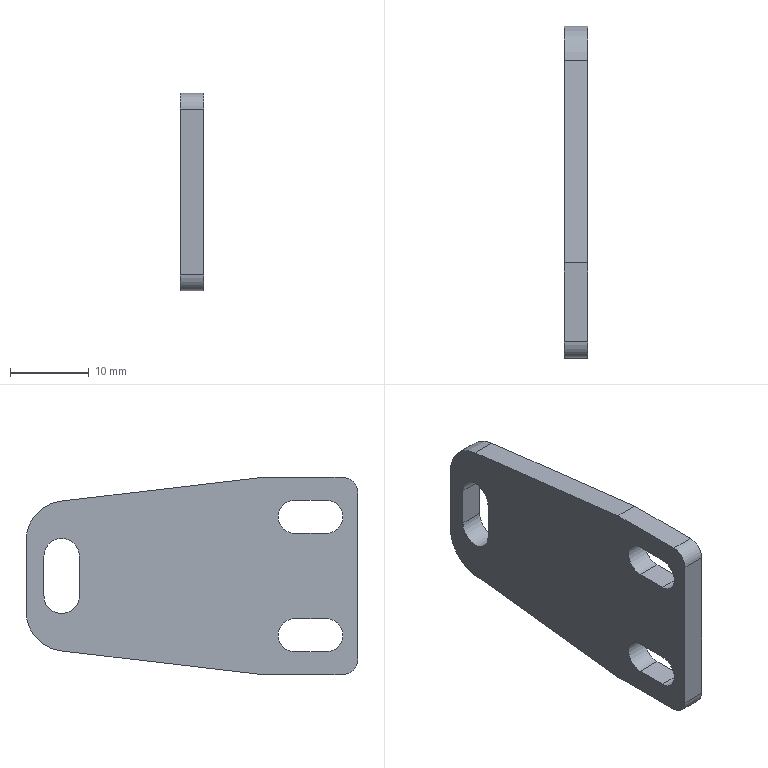Part | SolidWorks | features Fillet 3, ICE 3, Cut 1, Extrusion 1, HoleWzd 1 | 1 solid | 25 faces | box 3 x 42 x 25 mm | volume 2502 mm3 | plane 14 | cylinder 11 | commonest cylinder face diameters 4.2 x4 4.5 x3 4 x2 10 x2
STEP:
#1=CARTESIAN_POINT('',(3.,33.75,2.5));
#2=VERTEX_POINT('',#1);
#3=CARTESIAN_POINT('',(3.,31.5,4.75));
#4=VERTEX_POINT('',#3);
#5=CARTESIAN_POINT('',(3.,31.5,2.5));
#6=DIRECTION('',(1.,0.,0.));
#7=DIRECTION('',(0.,0.,-1.));
#8=AXIS2_PLACEMENT_3D('',#5,#6,#7);
#9=CIRCLE('',#8,2.25);
#10=EDGE_CURVE('',#2,#4,#9,.T.);
#11=ORIENTED_EDGE('',*,*,#10,.T.);
#12=CARTESIAN_POINT('',(0.,31.5,4.75));
#13=VERTEX_POINT('',#12);
#14=CARTESIAN_POINT('',(10.,31.5,4.75));
#15=DIRECTION('',(-1.,0.,0.));
#16=VECTOR('',#15,1000.);
#17=LINE('',#14,#16);
#18=EDGE_CURVE('',#4,#13,#17,.T.);
#19=ORIENTED_EDGE('',*,*,#18,.T.);
#20=CARTESIAN_POINT('',(0.,33.75,2.5));
#21=VERTEX_POINT('',#20);
#22=CARTESIAN_POINT('',(0.,31.5,2.5));
#23=DIRECTION('',(-1.,0.,0.));
#24=DIRECTION('',(0.,0.,1.));
#25=AXIS2_PLACEMENT_3D('',#22,#23,#24);
#26=CIRCLE('',#25,2.25);
#27=EDGE_CURVE('',#13,#21,#26,.T.);
#28=ORIENTED_EDGE('',*,*,#27,.T.);
#29=CARTESIAN_POINT('',(10.,33.75,2.5));
#30=DIRECTION('',(-1.,0.,0.));
#31=VECTOR('',#30,1000.);
#32=LINE('',#29,#31);
#33=EDGE_CURVE('',#2,#21,#32,.T.);
#34=ORIENTED_EDGE('',*,*,#33,.F.);
#35=EDGE_LOOP('',(#11,#19,#28,#34));
#36=FACE_OUTER_BOUND('',#35,.T.);
#37=CARTESIAN_POINT('',(10.,31.5,2.5));
#38=DIRECTION('',(-1.,0.,0.));
#39=DIRECTION('',(0.,0.,1.));
#40=AXIS2_PLACEMENT_3D('',#37,#38,#39);
#41=CYLINDRICAL_SURFACE('',#40,2.25);
#42=ADVANCED_FACE('',(#36),#41,.F.);
#43=CARTESIAN_POINT('',(0.,29.25,-2.5));
#44=VERTEX_POINT('',#43);
#45=CARTESIAN_POINT('',(0.,29.25,2.5));
#46=VERTEX_POINT('',#45);
#47=CARTESIAN_POINT('',(0.,29.25,-2.5));
#48=DIRECTION('',(0.,0.,1.));
#49=VECTOR('',#48,1000.);
#50=LINE('',#47,#49);
#51=EDGE_CURVE('',#44,#46,#50,.T.);
#52=ORIENTED_EDGE('',*,*,#51,.F.);
#53=CARTESIAN_POINT('',(0.,33.75,-2.5));
#54=VERTEX_POINT('',#53);
#55=CARTESIAN_POINT('',(0.,31.5,-2.5));
#56=DIRECTION('',(-1.,0.,0.));
#57=DIRECTION('',(0.,0.,1.));
#58=AXIS2_PLACEMENT_3D('',#55,#56,#57);
#59=CIRCLE('',#58,2.25);
#60=EDGE_CURVE('',#54,#44,#59,.T.);
#61=ORIENTED_EDGE('',*,*,#60,.F.);
#62=CARTESIAN_POINT('',(0.,33.75,-2.5));
#63=DIRECTION('',(0.,0.,-1.));
#64=VECTOR('',#63,1000.);
#65=LINE('',#62,#64);
#66=EDGE_CURVE('',#21,#54,#65,.T.);
#67=ORIENTED_EDGE('',*,*,#66,.F.);
#68=ORIENTED_EDGE('',*,*,#27,.F.);
#69=CARTESIAN_POINT('',(0.,31.5,2.5));
#70=DIRECTION('',(-1.,0.,0.));
#71=DIRECTION('',(0.,0.,1.));
#72=AXIS2_PLACEMENT_3D('',#69,#70,#71);
#73=CIRCLE('',#72,2.25);
#74=EDGE_CURVE('',#46,#13,#73,.T.);
#75=ORIENTED_EDGE('',*,*,#74,.F.);
#76=EDGE_LOOP('',(#52,#61,#67,#68,#75));
#77=FACE_BOUND('',#76,.T.);
#78=CARTESIAN_POINT('',(0.,2.,5.4));
#79=VERTEX_POINT('',#78);
#80=CARTESIAN_POINT('',(0.,-2.,5.4));
#81=VERTEX_POINT('',#80);
#82=CARTESIAN_POINT('',(0.,2.,5.4));
#83=DIRECTION('',(0.,-1.,0.));
#84=VECTOR('',#83,1000.);
#85=LINE('',#82,#84);
#86=EDGE_CURVE('',#79,#81,#85,.T.);
#87=ORIENTED_EDGE('',*,*,#86,.F.);
#88=CARTESIAN_POINT('',(0.,2.,9.6));
#89=VERTEX_POINT('',#88);
#90=CARTESIAN_POINT('',(0.,2.,7.5));
#91=DIRECTION('',(-1.,0.,0.));
#92=DIRECTION('',(0.,0.,-1.));
#93=AXIS2_PLACEMENT_3D('',#90,#91,#92);
#94=CIRCLE('',#93,2.1);
#95=EDGE_CURVE('',#89,#79,#94,.T.);
#96=ORIENTED_EDGE('',*,*,#95,.F.);
#97=CARTESIAN_POINT('',(0.,-2.,9.6));
#98=VERTEX_POINT('',#97);
#99=CARTESIAN_POINT('',(0.,2.,9.6));
#100=DIRECTION('',(0.,1.,0.));
#101=VECTOR('',#100,1000.);
#102=LINE('',#99,#101);
#103=EDGE_CURVE('',#98,#89,#102,.T.);
#104=ORIENTED_EDGE('',*,*,#103,.F.);
#105=CARTESIAN_POINT('',(0.,-2.,7.5));
#106=DIRECTION('',(-1.,0.,0.));
#107=DIRECTION('',(0.,0.,-1.));
#108=AXIS2_PLACEMENT_3D('',#105,#106,#107);
#109=CIRCLE('',#108,2.1);
#110=EDGE_CURVE('',#81,#98,#109,.T.);
#111=ORIENTED_EDGE('',*,*,#110,.F.);
#112=EDGE_LOOP('',(#87,#96,#104,#111));
#113=FACE_BOUND('',#112,.T.);
#114=CARTESIAN_POINT('',(0.,2.,-9.6));
#115=VERTEX_POINT('',#114);
#116=CARTESIAN_POINT('',(0.,-2.,-9.6));
#117=VERTEX_POINT('',#116);
#118=CARTESIAN_POINT('',(0.,2.,-9.6));
#119=DIRECTION('',(0.,-1.,0.));
#120=VECTOR('',#119,1000.);
#121=LINE('',#118,#120);
#122=EDGE_CURVE('',#115,#117,#121,.T.);
#123=ORIENTED_EDGE('',*,*,#122,.F.);
#124=CARTESIAN_POINT('',(0.,2.,-5.4));
#125=VERTEX_POINT('',#124);
#126=CARTESIAN_POINT('',(0.,2.,-7.5));
#127=DIRECTION('',(-1.,0.,0.));
#128=DIRECTION('',(0.,0.,1.));
#129=AXIS2_PLACEMENT_3D('',#126,#127,#128);
#130=CIRCLE('',#129,2.1);
#131=EDGE_CURVE('',#125,#115,#130,.T.);
#132=ORIENTED_EDGE('',*,*,#131,.F.);
#133=CARTESIAN_POINT('',(0.,-2.,-5.4));
#134=VERTEX_POINT('',#133);
#135=CARTESIAN_POINT('',(0.,2.,-5.4));
#136=DIRECTION('',(0.,1.,0.));
#137=VECTOR('',#136,1000.);
#138=LINE('',#135,#137);
#139=EDGE_CURVE('',#134,#125,#138,.T.);
#140=ORIENTED_EDGE('',*,*,#139,.F.);
#141=CARTESIAN_POINT('',(0.,-2.,-7.5));
#142=DIRECTION('',(-1.,0.,0.));
#143=DIRECTION('',(0.,0.,1.));
#144=AXIS2_PLACEMENT_3D('',#141,#142,#143);
#145=CIRCLE('',#144,2.1);
#146=EDGE_CURVE('',#117,#134,#145,.T.);
#147=ORIENTED_EDGE('',*,*,#146,.F.);
#148=EDGE_LOOP('',(#123,#132,#140,#147));
#149=FACE_BOUND('',#148,.T.);
#150=CARTESIAN_POINT('',(0.,36.,4.511));
#151=VERTEX_POINT('',#150);
#152=CARTESIAN_POINT('',(0.,36.,-4.511));
#153=VERTEX_POINT('',#152);
#154=CARTESIAN_POINT('',(0.,36.,0.));
#155=DIRECTION('',(0.,0.,-1.));
#156=VECTOR('',#155,1000.);
#157=LINE('',#154,#156);
#158=EDGE_CURVE('',#151,#153,#157,.T.);
#159=ORIENTED_EDGE('',*,*,#158,.T.);
#160=CARTESIAN_POINT('',(0.,31.587,-9.476));
#161=VERTEX_POINT('',#160);
#162=CARTESIAN_POINT('',(0.,31.,-4.511));
#163=DIRECTION('',(-1.,0.,0.));
#164=DIRECTION('',(0.,0.,-1.));
#165=AXIS2_PLACEMENT_3D('',#162,#163,#164);
#166=CIRCLE('',#165,5.);
#167=EDGE_CURVE('',#153,#161,#166,.T.);
#168=ORIENTED_EDGE('',*,*,#167,.T.);
#169=CARTESIAN_POINT('',(0.,6.,-12.5));
#170=VERTEX_POINT('',#169);
#171=CARTESIAN_POINT('',(0.,61.,-6.));
#172=DIRECTION('',(0.,-0.9931,-0.1174));
#173=VECTOR('',#172,1000.);
#174=LINE('',#171,#173);
#175=EDGE_CURVE('',#161,#170,#174,.T.);
#176=ORIENTED_EDGE('',*,*,#175,.T.);
#177=CARTESIAN_POINT('',(0.,-4.,-12.5));
#178=VERTEX_POINT('',#177);
#179=CARTESIAN_POINT('',(0.,6.,-12.5));
#180=DIRECTION('',(0.,1.,0.));
#181=VECTOR('',#180,1000.);
#182=LINE('',#179,#181);
#183=EDGE_CURVE('',#178,#170,#182,.T.);
#184=ORIENTED_EDGE('',*,*,#183,.F.);
#185=CARTESIAN_POINT('',(0.,-6.,-10.5));
#186=VERTEX_POINT('',#185);
#187=CARTESIAN_POINT('',(0.,-4.,-10.5));
#188=DIRECTION('',(-1.,0.,0.));
#189=DIRECTION('',(0.,0.,-1.));
#190=AXIS2_PLACEMENT_3D('',#187,#188,#189);
#191=CIRCLE('',#190,2.);
#192=EDGE_CURVE('',#178,#186,#191,.T.);
#193=ORIENTED_EDGE('',*,*,#192,.T.);
#194=CARTESIAN_POINT('',(0.,-6.,10.5));
#195=VERTEX_POINT('',#194);
#196=CARTESIAN_POINT('',(0.,-6.,12.5));
#197=DIRECTION('',(0.,0.,-1.));
#198=VECTOR('',#197,1000.);
#199=LINE('',#196,#198);
#200=EDGE_CURVE('',#195,#186,#199,.T.);
#201=ORIENTED_EDGE('',*,*,#200,.F.);
#202=CARTESIAN_POINT('',(0.,-4.,12.5));
#203=VERTEX_POINT('',#202);
#204=CARTESIAN_POINT('',(0.,-4.,10.5));
#205=DIRECTION('',(-1.,0.,0.));
#206=DIRECTION('',(0.,0.,-1.));
#207=AXIS2_PLACEMENT_3D('',#204,#205,#206);
#208=CIRCLE('',#207,2.);
#209=EDGE_CURVE('',#195,#203,#208,.T.);
#210=ORIENTED_EDGE('',*,*,#209,.T.);
#211=CARTESIAN_POINT('',(0.,6.,12.5));
#212=VERTEX_POINT('',#211);
#213=CARTESIAN_POINT('',(0.,6.,12.5));
#214=DIRECTION('',(0.,-1.,0.));
#215=VECTOR('',#214,1000.);
#216=LINE('',#213,#215);
#217=EDGE_CURVE('',#212,#203,#216,.T.);
#218=ORIENTED_EDGE('',*,*,#217,.F.);
#219=CARTESIAN_POINT('',(0.,31.587,9.476));
#220=VERTEX_POINT('',#219);
#221=CARTESIAN_POINT('',(0.,61.,6.));
#222=DIRECTION('',(0.,0.9931,-0.1174));
#223=VECTOR('',#222,1000.);
#224=LINE('',#221,#223);
#225=EDGE_CURVE('',#212,#220,#224,.T.);
#226=ORIENTED_EDGE('',*,*,#225,.T.);
#227=CARTESIAN_POINT('',(0.,31.,4.511));
#228=DIRECTION('',(-1.,0.,0.));
#229=DIRECTION('',(0.,0.,-1.));
#230=AXIS2_PLACEMENT_3D('',#227,#228,#229);
#231=CIRCLE('',#230,5.);
#232=EDGE_CURVE('',#220,#151,#231,.T.);
#233=ORIENTED_EDGE('',*,*,#232,.T.);
#234=EDGE_LOOP('',(#159,#168,#176,#184,#193,#201,#210,#218,#226,#233));
#235=FACE_OUTER_BOUND('',#234,.T.);
#236=CARTESIAN_POINT('',(0.,0.,0.));
#237=DIRECTION('',(1.,0.,0.));
#238=DIRECTION('',(0.,0.,-1.));
#239=AXIS2_PLACEMENT_3D('',#236,#237,#238);
#240=PLANE('',#239);
#241=ADVANCED_FACE('',(#77,#113,#149,#235),#240,.F.);
#242=CARTESIAN_POINT('',(3.,-4.,-12.5));
#243=VERTEX_POINT('',#242);
#244=CARTESIAN_POINT('',(3.,6.,-12.5));
#245=VERTEX_POINT('',#244);
#246=CARTESIAN_POINT('',(3.,6.,-12.5));
#247=DIRECTION('',(0.,1.,0.));
#248=VECTOR('',#247,1000.);
#249=LINE('',#246,#248);
#250=EDGE_CURVE('',#243,#245,#249,.T.);
#251=ORIENTED_EDGE('',*,*,#250,.F.);
#252=CARTESIAN_POINT('',(3.,-4.,-12.5));
#253=DIRECTION('',(-1.,0.,0.));
#254=VECTOR('',#253,1000.);
#255=LINE('',#252,#254);
#256=EDGE_CURVE('',#243,#178,#255,.T.);
#257=ORIENTED_EDGE('',*,*,#256,.T.);
#258=ORIENTED_EDGE('',*,*,#183,.T.);
#259=CARTESIAN_POINT('',(3.,6.,-12.5));
#260=DIRECTION('',(-1.,0.,0.));
#261=VECTOR('',#260,1000.);
#262=LINE('',#259,#261);
#263=EDGE_CURVE('',#245,#170,#262,.T.);
#264=ORIENTED_EDGE('',*,*,#263,.F.);
#265=EDGE_LOOP('',(#251,#257,#258,#264));
#266=FACE_OUTER_BOUND('',#265,.T.);
#267=CARTESIAN_POINT('',(3.,6.,-12.5));
#268=DIRECTION('',(0.,0.,1.));
#269=DIRECTION('',(0.,-1.,0.));
#270=AXIS2_PLACEMENT_3D('',#267,#268,#269);
#271=PLANE('',#270);
#272=ADVANCED_FACE('',(#266),#271,.F.);
#273=ORIENTED_EDGE('',*,*,#217,.T.);
#274=CARTESIAN_POINT('',(3.,-4.,12.5));
#275=VERTEX_POINT('',#274);
#276=CARTESIAN_POINT('',(3.,-4.,12.5));
#277=DIRECTION('',(1.,0.,0.));
#278=VECTOR('',#277,1000.);
#279=LINE('',#276,#278);
#280=EDGE_CURVE('',#203,#275,#279,.T.);
#281=ORIENTED_EDGE('',*,*,#280,.T.);
#282=CARTESIAN_POINT('',(3.,6.,12.5));
#283=VERTEX_POINT('',#282);
#284=CARTESIAN_POINT('',(3.,6.,12.5));
#285=DIRECTION('',(0.,-1.,0.));
#286=VECTOR('',#285,1000.);
#287=LINE('',#284,#286);
#288=EDGE_CURVE('',#283,#275,#287,.T.);
#289=ORIENTED_EDGE('',*,*,#288,.F.);
#290=CARTESIAN_POINT('',(3.,6.,12.5));
#291=DIRECTION('',(-1.,0.,0.));
#292=VECTOR('',#291,1000.);
#293=LINE('',#290,#292);
#294=EDGE_CURVE('',#283,#212,#293,.T.);
#295=ORIENTED_EDGE('',*,*,#294,.T.);
#296=EDGE_LOOP('',(#273,#281,#289,#295));
#297=FACE_OUTER_BOUND('',#296,.T.);
#298=CARTESIAN_POINT('',(3.,6.,12.5));
#299=DIRECTION('',(0.,0.,-1.));
#300=DIRECTION('',(-1.,0.,0.));
#301=AXIS2_PLACEMENT_3D('',#298,#299,#300);
#302=PLANE('',#301);
#303=ADVANCED_FACE('',(#297),#302,.F.);
#304=ORIENTED_EDGE('',*,*,#200,.T.);
#305=CARTESIAN_POINT('',(3.,-6.,-10.5));
#306=VERTEX_POINT('',#305);
#307=CARTESIAN_POINT('',(3.,-6.,-10.5));
#308=DIRECTION('',(1.,0.,0.));
#309=VECTOR('',#308,1000.);
#310=LINE('',#307,#309);
#311=EDGE_CURVE('',#186,#306,#310,.T.);
#312=ORIENTED_EDGE('',*,*,#311,.T.);
#313=CARTESIAN_POINT('',(3.,-6.,10.5));
#314=VERTEX_POINT('',#313);
#315=CARTESIAN_POINT('',(3.,-6.,12.5));
#316=DIRECTION('',(0.,0.,-1.));
#317=VECTOR('',#316,1000.);
#318=LINE('',#315,#317);
#319=EDGE_CURVE('',#314,#306,#318,.T.);
#320=ORIENTED_EDGE('',*,*,#319,.F.);
#321=CARTESIAN_POINT('',(3.,-6.,10.5));
#322=DIRECTION('',(-1.,0.,0.));
#323=VECTOR('',#322,1000.);
#324=LINE('',#321,#323);
#325=EDGE_CURVE('',#314,#195,#324,.T.);
#326=ORIENTED_EDGE('',*,*,#325,.T.);
#327=EDGE_LOOP('',(#304,#312,#320,#326));
#328=FACE_OUTER_BOUND('',#327,.T.);
#329=CARTESIAN_POINT('',(3.,-6.,12.5));
#330=DIRECTION('',(0.,1.,0.));
#331=DIRECTION('',(0.,0.,1.));
#332=AXIS2_PLACEMENT_3D('',#329,#330,#331);
#333=PLANE('',#332);
#334=ADVANCED_FACE('',(#328),#333,.F.);
#335=CARTESIAN_POINT('',(3.,29.25,-2.5));
#336=VERTEX_POINT('',#335);
#337=CARTESIAN_POINT('',(3.,33.75,-2.5));
#338=VERTEX_POINT('',#337);
#339=CARTESIAN_POINT('',(3.,31.5,-2.5));
#340=DIRECTION('',(1.,0.,0.));
#341=DIRECTION('',(0.,0.,-1.));
#342=AXIS2_PLACEMENT_3D('',#339,#340,#341);
#343=CIRCLE('',#342,2.25);
#344=EDGE_CURVE('',#336,#338,#343,.T.);
#345=ORIENTED_EDGE('',*,*,#344,.F.);
#346=CARTESIAN_POINT('',(3.,29.25,2.5));
#347=VERTEX_POINT('',#346);
#348=CARTESIAN_POINT('',(3.,29.25,0.));
#349=DIRECTION('',(0.,0.,-1.));
#350=VECTOR('',#349,1000.);
#351=LINE('',#348,#350);
#352=EDGE_CURVE('',#347,#336,#351,.T.);
#353=ORIENTED_EDGE('',*,*,#352,.F.);
#354=CARTESIAN_POINT('',(3.,31.5,2.5));
#355=DIRECTION('',(1.,0.,0.));
#356=DIRECTION('',(0.,0.,-1.));
#357=AXIS2_PLACEMENT_3D('',#354,#355,#356);
#358=CIRCLE('',#357,2.25);
#359=EDGE_CURVE('',#4,#347,#358,.T.);
#360=ORIENTED_EDGE('',*,*,#359,.F.);
#361=ORIENTED_EDGE('',*,*,#10,.F.);
#362=CARTESIAN_POINT('',(3.,33.75,0.));
#363=DIRECTION('',(0.,0.,1.));
#364=VECTOR('',#363,1000.);
#365=LINE('',#362,#364);
#366=EDGE_CURVE('',#338,#2,#365,.T.);
#367=ORIENTED_EDGE('',*,*,#366,.F.);
#368=EDGE_LOOP('',(#345,#353,#360,#361,#367));
#369=FACE_BOUND('',#368,.T.);
#370=CARTESIAN_POINT('',(3.,31.587,-9.476));
#371=VERTEX_POINT('',#370);
#372=CARTESIAN_POINT('',(3.,61.,-6.));
#373=DIRECTION('',(0.,-0.9931,-0.1174));
#374=VECTOR('',#373,1000.);
#375=LINE('',#372,#374);
#376=EDGE_CURVE('',#371,#245,#375,.T.);
#377=ORIENTED_EDGE('',*,*,#376,.F.);
#378=CARTESIAN_POINT('',(3.,36.,-4.511));
#379=VERTEX_POINT('',#378);
#380=CARTESIAN_POINT('',(3.,31.,-4.511));
#381=DIRECTION('',(1.,0.,0.));
#382=DIRECTION('',(0.,0.,-1.));
#383=AXIS2_PLACEMENT_3D('',#380,#381,#382);
#384=CIRCLE('',#383,5.);
#385=EDGE_CURVE('',#371,#379,#384,.T.);
#386=ORIENTED_EDGE('',*,*,#385,.T.);
#387=CARTESIAN_POINT('',(3.,36.,4.511));
#388=VERTEX_POINT('',#387);
#389=CARTESIAN_POINT('',(3.,36.,13.476));
#390=DIRECTION('',(0.,0.,-1.));
#391=VECTOR('',#390,1000.);
#392=LINE('',#389,#391);
#393=EDGE_CURVE('',#388,#379,#392,.T.);
#394=ORIENTED_EDGE('',*,*,#393,.F.);
#395=CARTESIAN_POINT('',(3.,31.587,9.476));
#396=VERTEX_POINT('',#395);
#397=CARTESIAN_POINT('',(3.,31.,4.511));
#398=DIRECTION('',(1.,0.,0.));
#399=DIRECTION('',(0.,0.,-1.));
#400=AXIS2_PLACEMENT_3D('',#397,#398,#399);
#401=CIRCLE('',#400,5.);
#402=EDGE_CURVE('',#388,#396,#401,.T.);
#403=ORIENTED_EDGE('',*,*,#402,.T.);
#404=CARTESIAN_POINT('',(3.,61.,6.));
#405=DIRECTION('',(0.,0.9931,-0.1174));
#406=VECTOR('',#405,1000.);
#407=LINE('',#404,#406);
#408=EDGE_CURVE('',#283,#396,#407,.T.);
#409=ORIENTED_EDGE('',*,*,#408,.F.);
#410=ORIENTED_EDGE('',*,*,#288,.T.);
#411=CARTESIAN_POINT('',(3.,-4.,10.5));
#412=DIRECTION('',(1.,0.,0.));
#413=DIRECTION('',(0.,0.,-1.));
#414=AXIS2_PLACEMENT_3D('',#411,#412,#413);
#415=CIRCLE('',#414,2.);
#416=EDGE_CURVE('',#275,#314,#415,.T.);
#417=ORIENTED_EDGE('',*,*,#416,.T.);
#418=ORIENTED_EDGE('',*,*,#319,.T.);
#419=CARTESIAN_POINT('',(3.,-4.,-10.5));
#420=DIRECTION('',(1.,0.,0.));
#421=DIRECTION('',(0.,0.,-1.));
#422=AXIS2_PLACEMENT_3D('',#419,#420,#421);
#423=CIRCLE('',#422,2.);
#424=EDGE_CURVE('',#306,#243,#423,.T.);
#425=ORIENTED_EDGE('',*,*,#424,.T.);
#426=ORIENTED_EDGE('',*,*,#250,.T.);
#427=EDGE_LOOP('',(#377,#386,#394,#403,#409,#410,#417,#418,#425,#426));
#428=FACE_OUTER_BOUND('',#427,.T.);
#429=CARTESIAN_POINT('',(3.,2.,9.6));
#430=VERTEX_POINT('',#429);
#431=CARTESIAN_POINT('',(3.,2.,5.4));
#432=VERTEX_POINT('',#431);
#433=CARTESIAN_POINT('',(3.,2.,7.5));
#434=DIRECTION('',(-1.,0.,0.));
#435=DIRECTION('',(0.,0.,-1.));
#436=AXIS2_PLACEMENT_3D('',#433,#434,#435);
#437=CIRCLE('',#436,2.1);
#438=EDGE_CURVE('',#430,#432,#437,.T.);
#439=ORIENTED_EDGE('',*,*,#438,.T.);
#440=CARTESIAN_POINT('',(3.,-2.,5.4));
#441=VERTEX_POINT('',#440);
#442=CARTESIAN_POINT('',(3.,2.,5.4));
#443=DIRECTION('',(0.,-1.,0.));
#444=VECTOR('',#443,1000.);
#445=LINE('',#442,#444);
#446=EDGE_CURVE('',#432,#441,#445,.T.);
#447=ORIENTED_EDGE('',*,*,#446,.T.);
#448=CARTESIAN_POINT('',(3.,-2.,9.6));
#449=VERTEX_POINT('',#448);
#450=CARTESIAN_POINT('',(3.,-2.,7.5));
#451=DIRECTION('',(-1.,0.,0.));
#452=DIRECTION('',(0.,0.,-1.));
#453=AXIS2_PLACEMENT_3D('',#450,#451,#452);
#454=CIRCLE('',#453,2.1);
#455=EDGE_CURVE('',#441,#449,#454,.T.);
#456=ORIENTED_EDGE('',*,*,#455,.T.);
#457=CARTESIAN_POINT('',(3.,2.,9.6));
#458=DIRECTION('',(0.,1.,0.));
#459=VECTOR('',#458,1000.);
#460=LINE('',#457,#459);
#461=EDGE_CURVE('',#449,#430,#460,.T.);
#462=ORIENTED_EDGE('',*,*,#461,.T.);
#463=EDGE_LOOP('',(#439,#447,#456,#462));
#464=FACE_BOUND('',#463,.T.);
#465=CARTESIAN_POINT('',(3.,2.,-5.4));
#466=VERTEX_POINT('',#465);
#467=CARTESIAN_POINT('',(3.,2.,-9.6));
#468=VERTEX_POINT('',#467);
#469=CARTESIAN_POINT('',(3.,2.,-7.5));
#470=DIRECTION('',(-1.,0.,0.));
#471=DIRECTION('',(0.,0.,1.));
#472=AXIS2_PLACEMENT_3D('',#469,#470,#471);
#473=CIRCLE('',#472,2.1);
#474=EDGE_CURVE('',#466,#468,#473,.T.);
#475=ORIENTED_EDGE('',*,*,#474,.T.);
#476=CARTESIAN_POINT('',(3.,-2.,-9.6));
#477=VERTEX_POINT('',#476);
#478=CARTESIAN_POINT('',(3.,2.,-9.6));
#479=DIRECTION('',(0.,-1.,0.));
#480=VECTOR('',#479,1000.);
#481=LINE('',#478,#480);
#482=EDGE_CURVE('',#468,#477,#481,.T.);
#483=ORIENTED_EDGE('',*,*,#482,.T.);
#484=CARTESIAN_POINT('',(3.,-2.,-5.4));
#485=VERTEX_POINT('',#484);
#486=CARTESIAN_POINT('',(3.,-2.,-7.5));
#487=DIRECTION('',(-1.,0.,0.));
#488=DIRECTION('',(0.,0.,1.));
#489=AXIS2_PLACEMENT_3D('',#486,#487,#488);
#490=CIRCLE('',#489,2.1);
#491=EDGE_CURVE('',#477,#485,#490,.T.);
#492=ORIENTED_EDGE('',*,*,#491,.T.);
#493=CARTESIAN_POINT('',(3.,2.,-5.4));
#494=DIRECTION('',(0.,1.,0.));
#495=VECTOR('',#494,1000.);
#496=LINE('',#493,#495);
#497=EDGE_CURVE('',#485,#466,#496,.T.);
#498=ORIENTED_EDGE('',*,*,#497,.T.);
#499=EDGE_LOOP('',(#475,#483,#492,#498));
#500=FACE_BOUND('',#499,.T.);
#501=CARTESIAN_POINT('',(3.,0.,0.));
#502=DIRECTION('',(1.,0.,0.));
#503=DIRECTION('',(0.,0.,-1.));
#504=AXIS2_PLACEMENT_3D('',#501,#502,#503);
#505=PLANE('',#504);
#506=ADVANCED_FACE('',(#369,#428,#464,#500),#505,.T.);
#507=ORIENTED_EDGE('',*,*,#175,.F.);
#508=CARTESIAN_POINT('',(3.,31.587,-9.476));
#509=DIRECTION('',(1.,0.,0.));
#510=VECTOR('',#509,1000.);
#511=LINE('',#508,#510);
#512=EDGE_CURVE('',#161,#371,#511,.T.);
#513=ORIENTED_EDGE('',*,*,#512,.T.);
#514=ORIENTED_EDGE('',*,*,#376,.T.);
#515=ORIENTED_EDGE('',*,*,#263,.T.);
#516=EDGE_LOOP('',(#507,#513,#514,#515));
#517=FACE_OUTER_BOUND('',#516,.T.);
#518=CARTESIAN_POINT('',(63.415,61.,-6.));
#519=DIRECTION('',(0.,0.1174,-0.9931));
#520=DIRECTION('',(0.,0.9931,0.1174));
#521=AXIS2_PLACEMENT_3D('',#518,#519,#520);
#522=PLANE('',#521);
#523=ADVANCED_FACE('',(#517),#522,.T.);
#524=ORIENTED_EDGE('',*,*,#408,.T.);
#525=CARTESIAN_POINT('',(0.,31.587,9.476));
#526=DIRECTION('',(-1.,0.,0.));
#527=VECTOR('',#526,1000.);
#528=LINE('',#525,#527);
#529=EDGE_CURVE('',#396,#220,#528,.T.);
#530=ORIENTED_EDGE('',*,*,#529,.T.);
#531=ORIENTED_EDGE('',*,*,#225,.F.);
#532=ORIENTED_EDGE('',*,*,#294,.F.);
#533=EDGE_LOOP('',(#524,#530,#531,#532));
#534=FACE_OUTER_BOUND('',#533,.T.);
#535=CARTESIAN_POINT('',(63.415,61.,6.));
#536=DIRECTION('',(0.,0.1174,0.9931));
#537=DIRECTION('',(0.,-0.9931,0.1174));
#538=AXIS2_PLACEMENT_3D('',#535,#536,#537);
#539=PLANE('',#538);
#540=ADVANCED_FACE('',(#534),#539,.T.);
#541=ORIENTED_EDGE('',*,*,#131,.T.);
#542=CARTESIAN_POINT('',(3.,2.,-9.6));
#543=DIRECTION('',(-1.,0.,0.));
#544=VECTOR('',#543,1000.);
#545=LINE('',#542,#544);
#546=EDGE_CURVE('',#468,#115,#545,.T.);
#547=ORIENTED_EDGE('',*,*,#546,.F.);
#548=ORIENTED_EDGE('',*,*,#474,.F.);
#549=CARTESIAN_POINT('',(3.,2.,-5.4));
#550=DIRECTION('',(-1.,0.,0.));
#551=VECTOR('',#550,1000.);
#552=LINE('',#549,#551);
#553=EDGE_CURVE('',#466,#125,#552,.T.);
#554=ORIENTED_EDGE('',*,*,#553,.T.);
#555=EDGE_LOOP('',(#541,#547,#548,#554));
#556=FACE_OUTER_BOUND('',#555,.T.);
#557=CARTESIAN_POINT('',(3.,2.,-7.5));
#558=DIRECTION('',(-1.,0.,0.));
#559=DIRECTION('',(0.,0.,1.));
#560=AXIS2_PLACEMENT_3D('',#557,#558,#559);
#561=CYLINDRICAL_SURFACE('',#560,2.1);
#562=ADVANCED_FACE('',(#556),#561,.F.);
#563=ORIENTED_EDGE('',*,*,#139,.T.);
#564=ORIENTED_EDGE('',*,*,#553,.F.);
#565=ORIENTED_EDGE('',*,*,#497,.F.);
#566=CARTESIAN_POINT('',(3.,-2.,-5.4));
#567=DIRECTION('',(-1.,0.,0.));
#568=VECTOR('',#567,1000.);
#569=LINE('',#566,#568);
#570=EDGE_CURVE('',#485,#134,#569,.T.);
#571=ORIENTED_EDGE('',*,*,#570,.T.);
#572=EDGE_LOOP('',(#563,#564,#565,#571));
#573=FACE_OUTER_BOUND('',#572,.T.);
#574=CARTESIAN_POINT('',(3.,2.,-5.4));
#575=DIRECTION('',(0.,0.,1.));
#576=DIRECTION('',(1.,0.,0.));
#577=AXIS2_PLACEMENT_3D('',#574,#575,#576);
#578=PLANE('',#577);
#579=ADVANCED_FACE('',(#573),#578,.F.);
#580=ORIENTED_EDGE('',*,*,#146,.T.);
#581=ORIENTED_EDGE('',*,*,#570,.F.);
#582=ORIENTED_EDGE('',*,*,#491,.F.);
#583=CARTESIAN_POINT('',(3.,-2.,-9.6));
#584=DIRECTION('',(-1.,0.,0.));
#585=VECTOR('',#584,1000.);
#586=LINE('',#583,#585);
#587=EDGE_CURVE('',#477,#117,#586,.T.);
#588=ORIENTED_EDGE('',*,*,#587,.T.);
#589=EDGE_LOOP('',(#580,#581,#582,#588));
#590=FACE_OUTER_BOUND('',#589,.T.);
#591=CARTESIAN_POINT('',(3.,-2.,-7.5));
#592=DIRECTION('',(-1.,0.,0.));
#593=DIRECTION('',(0.,0.,1.));
#594=AXIS2_PLACEMENT_3D('',#591,#592,#593);
#595=CYLINDRICAL_SURFACE('',#594,2.1);
#596=ADVANCED_FACE('',(#590),#595,.F.);
#597=ORIENTED_EDGE('',*,*,#122,.T.);
#598=ORIENTED_EDGE('',*,*,#587,.F.);
#599=ORIENTED_EDGE('',*,*,#482,.F.);
#600=ORIENTED_EDGE('',*,*,#546,.T.);
#601=EDGE_LOOP('',(#597,#598,#599,#600));
#602=FACE_OUTER_BOUND('',#601,.T.);
#603=CARTESIAN_POINT('',(3.,2.,-9.6));
#604=DIRECTION('',(0.,0.,-1.));
#605=DIRECTION('',(-1.,0.,0.));
#606=AXIS2_PLACEMENT_3D('',#603,#604,#605);
#607=PLANE('',#606);
#608=ADVANCED_FACE('',(#602),#607,.F.);
#609=ORIENTED_EDGE('',*,*,#95,.T.);
#610=CARTESIAN_POINT('',(3.,2.,5.4));
#611=DIRECTION('',(-1.,0.,0.));
#612=VECTOR('',#611,1000.);
#613=LINE('',#610,#612);
#614=EDGE_CURVE('',#432,#79,#613,.T.);
#615=ORIENTED_EDGE('',*,*,#614,.F.);
#616=ORIENTED_EDGE('',*,*,#438,.F.);
#617=CARTESIAN_POINT('',(3.,2.,9.6));
#618=DIRECTION('',(-1.,0.,0.));
#619=VECTOR('',#618,1000.);
#620=LINE('',#617,#619);
#621=EDGE_CURVE('',#430,#89,#620,.T.);
#622=ORIENTED_EDGE('',*,*,#621,.T.);
#623=EDGE_LOOP('',(#609,#615,#616,#622));
#624=FACE_OUTER_BOUND('',#623,.T.);
#625=CARTESIAN_POINT('',(3.,2.,7.5));
#626=DIRECTION('',(-1.,0.,0.));
#627=DIRECTION('',(0.,0.,1.));
#628=AXIS2_PLACEMENT_3D('',#625,#626,#627);
#629=CYLINDRICAL_SURFACE('',#628,2.1);
#630=ADVANCED_FACE('',(#624),#629,.F.);
#631=ORIENTED_EDGE('',*,*,#103,.T.);
#632=ORIENTED_EDGE('',*,*,#621,.F.);
#633=ORIENTED_EDGE('',*,*,#461,.F.);
#634=CARTESIAN_POINT('',(3.,-2.,9.6));
#635=DIRECTION('',(-1.,0.,0.));
#636=VECTOR('',#635,1000.);
#637=LINE('',#634,#636);
#638=EDGE_CURVE('',#449,#98,#637,.T.);
#639=ORIENTED_EDGE('',*,*,#638,.T.);
#640=EDGE_LOOP('',(#631,#632,#633,#639));
#641=FACE_OUTER_BOUND('',#640,.T.);
#642=CARTESIAN_POINT('',(3.,2.,9.6));
#643=DIRECTION('',(0.,0.,1.));
#644=DIRECTION('',(1.,0.,0.));
#645=AXIS2_PLACEMENT_3D('',#642,#643,#644);
#646=PLANE('',#645);
#647=ADVANCED_FACE('',(#641),#646,.F.);
#648=ORIENTED_EDGE('',*,*,#110,.T.);
#649=ORIENTED_EDGE('',*,*,#638,.F.);
#650=ORIENTED_EDGE('',*,*,#455,.F.);
#651=CARTESIAN_POINT('',(3.,-2.,5.4));
#652=DIRECTION('',(-1.,0.,0.));
#653=VECTOR('',#652,1000.);
#654=LINE('',#651,#653);
#655=EDGE_CURVE('',#441,#81,#654,.T.);
#656=ORIENTED_EDGE('',*,*,#655,.T.);
#657=EDGE_LOOP('',(#648,#649,#650,#656));
#658=FACE_OUTER_BOUND('',#657,.T.);
#659=CARTESIAN_POINT('',(3.,-2.,7.5));
#660=DIRECTION('',(-1.,0.,0.));
#661=DIRECTION('',(0.,0.,1.));
#662=AXIS2_PLACEMENT_3D('',#659,#660,#661);
#663=CYLINDRICAL_SURFACE('',#662,2.1);
#664=ADVANCED_FACE('',(#658),#663,.F.);
#665=ORIENTED_EDGE('',*,*,#86,.T.);
#666=ORIENTED_EDGE('',*,*,#655,.F.);
#667=ORIENTED_EDGE('',*,*,#446,.F.);
#668=ORIENTED_EDGE('',*,*,#614,.T.);
#669=EDGE_LOOP('',(#665,#666,#667,#668));
#670=FACE_OUTER_BOUND('',#669,.T.);
#671=CARTESIAN_POINT('',(3.,2.,5.4));
#672=DIRECTION('',(0.,0.,-1.));
#673=DIRECTION('',(-1.,0.,0.));
#674=AXIS2_PLACEMENT_3D('',#671,#672,#673);
#675=PLANE('',#674);
#676=ADVANCED_FACE('',(#670),#675,.F.);
#677=ORIENTED_EDGE('',*,*,#424,.F.);
#678=ORIENTED_EDGE('',*,*,#311,.F.);
#679=ORIENTED_EDGE('',*,*,#192,.F.);
#680=ORIENTED_EDGE('',*,*,#256,.F.);
#681=EDGE_LOOP('',(#677,#678,#679,#680));
#682=FACE_OUTER_BOUND('',#681,.T.);
#683=CARTESIAN_POINT('',(3.,-4.,-10.5));
#684=DIRECTION('',(-1.,0.,0.));
#685=DIRECTION('',(0.,0.,1.));
#686=AXIS2_PLACEMENT_3D('',#683,#684,#685);
#687=CYLINDRICAL_SURFACE('',#686,2.);
#688=ADVANCED_FACE('',(#682),#687,.T.);
#689=ORIENTED_EDGE('',*,*,#416,.F.);
#690=ORIENTED_EDGE('',*,*,#280,.F.);
#691=ORIENTED_EDGE('',*,*,#209,.F.);
#692=ORIENTED_EDGE('',*,*,#325,.F.);
#693=EDGE_LOOP('',(#689,#690,#691,#692));
#694=FACE_OUTER_BOUND('',#693,.T.);
#695=CARTESIAN_POINT('',(3.,-4.,10.5));
#696=DIRECTION('',(-1.,0.,0.));
#697=DIRECTION('',(0.,0.,1.));
#698=AXIS2_PLACEMENT_3D('',#695,#696,#697);
#699=CYLINDRICAL_SURFACE('',#698,2.);
#700=ADVANCED_FACE('',(#694),#699,.T.);
#701=ORIENTED_EDGE('',*,*,#393,.T.);
#702=CARTESIAN_POINT('',(0.,36.,-4.511));
#703=DIRECTION('',(-1.,0.,0.));
#704=VECTOR('',#703,1000.);
#705=LINE('',#702,#704);
#706=EDGE_CURVE('',#379,#153,#705,.T.);
#707=ORIENTED_EDGE('',*,*,#706,.T.);
#708=ORIENTED_EDGE('',*,*,#158,.F.);
#709=CARTESIAN_POINT('',(3.,36.,4.511));
#710=DIRECTION('',(1.,0.,0.));
#711=VECTOR('',#710,1000.);
#712=LINE('',#709,#711);
#713=EDGE_CURVE('',#151,#388,#712,.T.);
#714=ORIENTED_EDGE('',*,*,#713,.T.);
#715=EDGE_LOOP('',(#701,#707,#708,#714));
#716=FACE_OUTER_BOUND('',#715,.T.);
#717=CARTESIAN_POINT('',(-7.,36.,13.476));
#718=DIRECTION('',(0.,-1.,0.));
#719=DIRECTION('',(0.,0.,-1.));
#720=AXIS2_PLACEMENT_3D('',#717,#718,#719);
#721=PLANE('',#720);
#722=ADVANCED_FACE('',(#716),#721,.F.);
#723=ORIENTED_EDGE('',*,*,#344,.T.);
#724=CARTESIAN_POINT('',(10.,33.75,-2.5));
#725=DIRECTION('',(-1.,0.,0.));
#726=VECTOR('',#725,1000.);
#727=LINE('',#724,#726);
#728=EDGE_CURVE('',#338,#54,#727,.T.);
#729=ORIENTED_EDGE('',*,*,#728,.T.);
#730=ORIENTED_EDGE('',*,*,#60,.T.);
#731=CARTESIAN_POINT('',(10.,29.25,-2.5));
#732=DIRECTION('',(-1.,0.,0.));
#733=VECTOR('',#732,1000.);
#734=LINE('',#731,#733);
#735=EDGE_CURVE('',#336,#44,#734,.T.);
#736=ORIENTED_EDGE('',*,*,#735,.F.);
#737=EDGE_LOOP('',(#723,#729,#730,#736));
#738=FACE_OUTER_BOUND('',#737,.T.);
#739=CARTESIAN_POINT('',(10.,31.5,-2.5));
#740=DIRECTION('',(-1.,0.,0.));
#741=DIRECTION('',(0.,0.,1.));
#742=AXIS2_PLACEMENT_3D('',#739,#740,#741);
#743=CYLINDRICAL_SURFACE('',#742,2.25);
#744=ADVANCED_FACE('',(#738),#743,.F.);
#745=ORIENTED_EDGE('',*,*,#366,.T.);
#746=ORIENTED_EDGE('',*,*,#33,.T.);
#747=ORIENTED_EDGE('',*,*,#66,.T.);
#748=ORIENTED_EDGE('',*,*,#728,.F.);
#749=EDGE_LOOP('',(#745,#746,#747,#748));
#750=FACE_OUTER_BOUND('',#749,.T.);
#751=CARTESIAN_POINT('',(10.,33.75,-2.5));
#752=DIRECTION('',(0.,1.,0.));
#753=DIRECTION('',(0.,0.,1.));
#754=AXIS2_PLACEMENT_3D('',#751,#752,#753);
#755=PLANE('',#754);
#756=ADVANCED_FACE('',(#750),#755,.F.);
#757=ORIENTED_EDGE('',*,*,#18,.F.);
#758=ORIENTED_EDGE('',*,*,#359,.T.);
#759=CARTESIAN_POINT('',(10.,29.25,2.5));
#760=DIRECTION('',(-1.,0.,0.));
#761=VECTOR('',#760,1000.);
#762=LINE('',#759,#761);
#763=EDGE_CURVE('',#347,#46,#762,.T.);
#764=ORIENTED_EDGE('',*,*,#763,.T.);
#765=ORIENTED_EDGE('',*,*,#74,.T.);
#766=EDGE_LOOP('',(#757,#758,#764,#765));
#767=FACE_OUTER_BOUND('',#766,.T.);
#768=CARTESIAN_POINT('',(10.,31.5,2.5));
#769=DIRECTION('',(-1.,0.,0.));
#770=DIRECTION('',(0.,0.,1.));
#771=AXIS2_PLACEMENT_3D('',#768,#769,#770);
#772=CYLINDRICAL_SURFACE('',#771,2.25);
#773=ADVANCED_FACE('',(#767),#772,.F.);
#774=ORIENTED_EDGE('',*,*,#352,.T.);
#775=ORIENTED_EDGE('',*,*,#735,.T.);
#776=ORIENTED_EDGE('',*,*,#51,.T.);
#777=ORIENTED_EDGE('',*,*,#763,.F.);
#778=EDGE_LOOP('',(#774,#775,#776,#777));
#779=FACE_OUTER_BOUND('',#778,.T.);
#780=CARTESIAN_POINT('',(10.,29.25,-2.5));
#781=DIRECTION('',(0.,-1.,0.));
#782=DIRECTION('',(0.,0.,-1.));
#783=AXIS2_PLACEMENT_3D('',#780,#781,#782);
#784=PLANE('',#783);
#785=ADVANCED_FACE('',(#779),#784,.F.);
#786=ORIENTED_EDGE('',*,*,#385,.F.);
#787=ORIENTED_EDGE('',*,*,#512,.F.);
#788=ORIENTED_EDGE('',*,*,#167,.F.);
#789=ORIENTED_EDGE('',*,*,#706,.F.);
#790=EDGE_LOOP('',(#786,#787,#788,#789));
#791=FACE_OUTER_BOUND('',#790,.T.);
#792=CARTESIAN_POINT('',(-7.,31.,-4.511));
#793=DIRECTION('',(1.,0.,0.));
#794=DIRECTION('',(0.,0.,-1.));
#795=AXIS2_PLACEMENT_3D('',#792,#793,#794);
#796=CYLINDRICAL_SURFACE('',#795,5.);
#797=ADVANCED_FACE('',(#791),#796,.T.);
#798=ORIENTED_EDGE('',*,*,#232,.F.);
#799=ORIENTED_EDGE('',*,*,#529,.F.);
#800=ORIENTED_EDGE('',*,*,#402,.F.);
#801=ORIENTED_EDGE('',*,*,#713,.F.);
#802=EDGE_LOOP('',(#798,#799,#800,#801));
#803=FACE_OUTER_BOUND('',#802,.T.);
#804=CARTESIAN_POINT('',(-7.,31.,4.511));
#805=DIRECTION('',(-1.,0.,0.));
#806=DIRECTION('',(0.,0.,1.));
#807=AXIS2_PLACEMENT_3D('',#804,#805,#806);
#808=CYLINDRICAL_SURFACE('',#807,5.);
#809=ADVANCED_FACE('',(#803),#808,.T.);
#810=CLOSED_SHELL('',(#42,#241,#272,#303,#334,#506,#523,#540,#562,#579,#596,#608,#630,#647,#664,#676,#688,#700,#722,#744,#756,#773,#785,#797,#809));
#811=MANIFOLD_SOLID_BREP('',#810);
#812=CARTESIAN_POINT('',(0.,0.,0.));
#813=DIRECTION('',(0.,0.,1.));
#814=DIRECTION('',(1.,0.,0.));
#815=AXIS2_PLACEMENT_3D('',#812,#813,#814);
#816=(LENGTH_UNIT()NAMED_UNIT(*)SI_UNIT(.MILLI.,.METRE.));
#817=UNCERTAINTY_MEASURE_WITH_UNIT(LENGTH_MEASURE(0.00001),#816,'','');
#818=(NAMED_UNIT(*)PLANE_ANGLE_UNIT()SI_UNIT($,.RADIAN.));
#819=(NAMED_UNIT(*)SI_UNIT($,.STERADIAN.)SOLID_ANGLE_UNIT());
#820=(GEOMETRIC_REPRESENTATION_CONTEXT(3)GLOBAL_UNCERTAINTY_ASSIGNED_CONTEXT((#817))GLOBAL_UNIT_ASSIGNED_CONTEXT((#816,#818,#819))REPRESENTATION_CONTEXT('',''));
#821=ADVANCED_BREP_SHAPE_REPRESENTATION('',(#811,#815),#820);